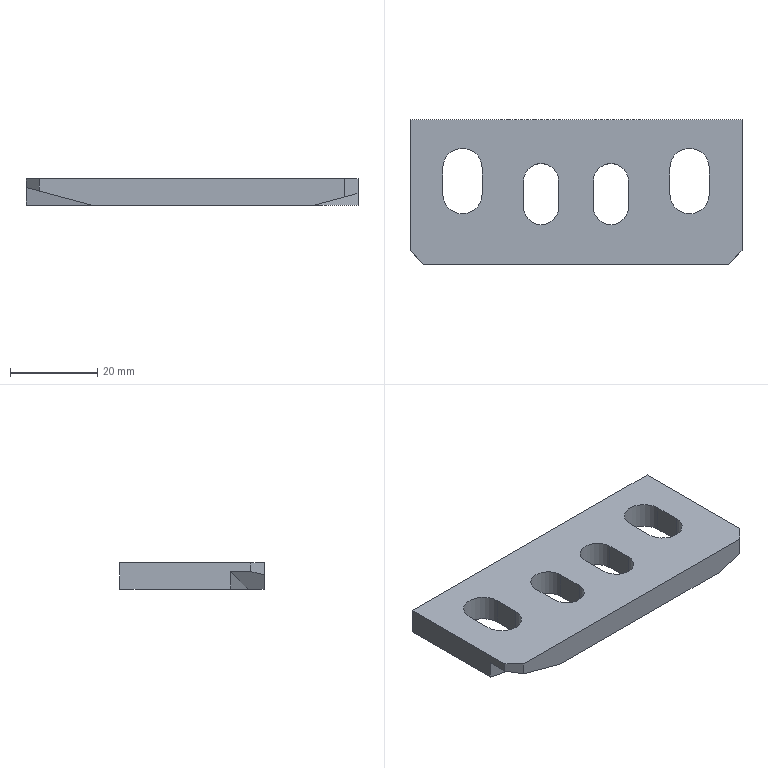Part | STEP file | gslz 2016.10.28-13_id1582_x_t | 1 solid | 29 faces | box 76 x 33 x 6 mm | volume 12149 mm3 | plane 21 | cylinder 8 | commonest cylinder face diameters 8 x4 9 x4